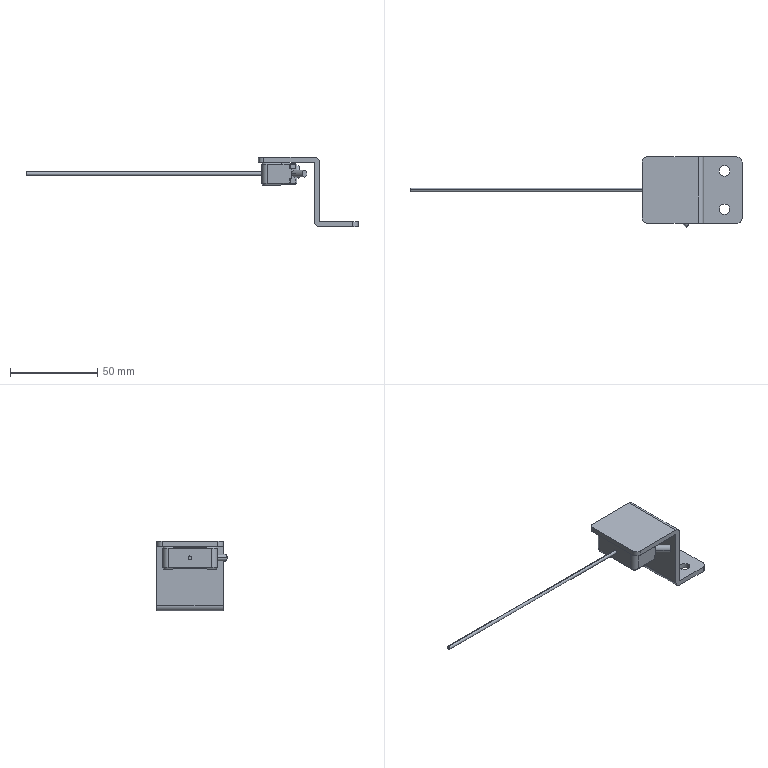Part | SolidWorks | 3 solids | 233 faces | box 190 x 40.32 x 40 mm | volume 18095 mm3 | plane 123 | cylinder 95 | cone 15 | commonest cylinder face diameters 0.3 x25 0.5 x22 6 x16 2.5 x6 0.2 x5 1 x4